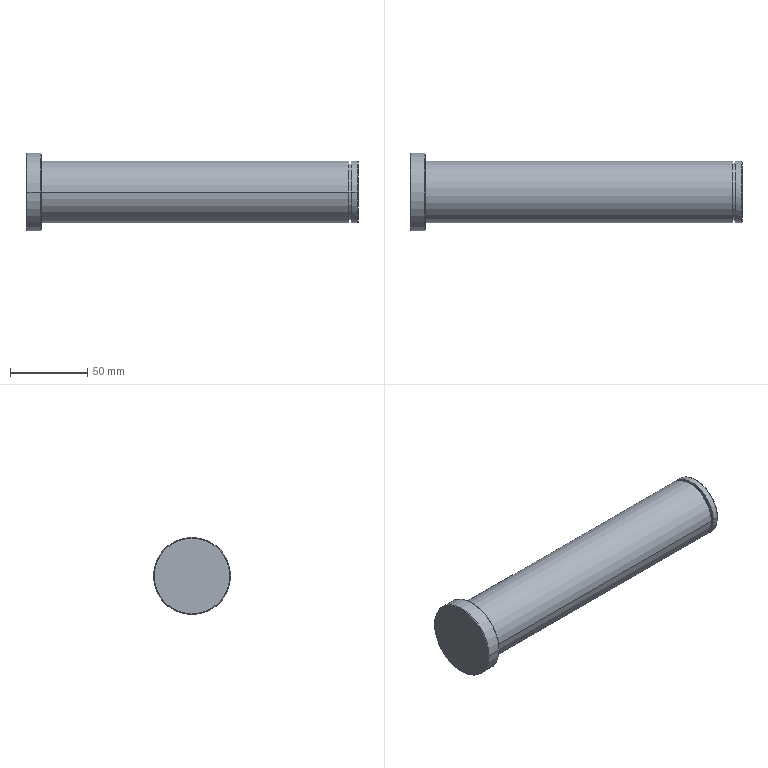Part | SolidWorks | features BaseBody 1 | 1 solid | 19 faces | box 215 x 50 x 50 mm | volume 276823 mm3 | cylinder 8 | cone 6 | plane 5 | commonest cylinder face diameters 40 x4 36.5 x2 50 x2
STEP:
#1=CARTESIAN_POINT('',(24.077,-7.842,0.));
#2=VERTEX_POINT('',#1);
#3=CARTESIAN_POINT('',(24.077,-47.842,0.));
#4=VERTEX_POINT('',#3);
#5=CARTESIAN_POINT('',(24.077,-27.842,0.));
#6=DIRECTION('',(1.,0.,0.));
#7=DIRECTION('',(0.,1.,0.));
#8=AXIS2_PLACEMENT_3D('',#5,#6,#7);
#9=CIRCLE('',#8,20.);
#10=EDGE_CURVE('',#2,#4,#9,.T.);
#11=ORIENTED_EDGE('',*,*,#10,.T.);
#12=CARTESIAN_POINT('',(223.077,-47.842,0.));
#13=VERTEX_POINT('',#12);
#14=CARTESIAN_POINT('',(123.577,-47.842,0.));
#15=DIRECTION('',(1.,0.,0.));
#16=VECTOR('',#15,1000.);
#17=LINE('',#14,#16);
#18=EDGE_CURVE('',#4,#13,#17,.T.);
#19=ORIENTED_EDGE('',*,*,#18,.T.);
#20=CARTESIAN_POINT('',(223.077,-7.842,0.));
#21=VERTEX_POINT('',#20);
#22=CARTESIAN_POINT('',(223.077,-27.842,0.));
#23=DIRECTION('',(-1.,0.,0.));
#24=DIRECTION('',(0.,1.,0.));
#25=AXIS2_PLACEMENT_3D('',#22,#23,#24);
#26=CIRCLE('',#25,20.);
#27=EDGE_CURVE('',#13,#21,#26,.T.);
#28=ORIENTED_EDGE('',*,*,#27,.T.);
#29=CARTESIAN_POINT('',(123.577,-7.842,0.));
#30=DIRECTION('',(1.,0.,0.));
#31=VECTOR('',#30,1000.);
#32=LINE('',#29,#31);
#33=EDGE_CURVE('',#2,#21,#32,.T.);
#34=ORIENTED_EDGE('',*,*,#33,.F.);
#35=EDGE_LOOP('',(#11,#19,#28,#34));
#36=FACE_OUTER_BOUND('',#35,.T.);
#37=CARTESIAN_POINT('',(123.577,-27.842,0.));
#38=DIRECTION('',(1.,0.,0.));
#39=DIRECTION('',(0.,1.,0.));
#40=AXIS2_PLACEMENT_3D('',#37,#38,#39);
#41=CYLINDRICAL_SURFACE('',#40,20.);
#42=ADVANCED_FACE('',(#36),#41,.T.);
#43=CARTESIAN_POINT('',(24.077,-27.842,-24.5));
#44=VERTEX_POINT('',#43);
#45=CARTESIAN_POINT('',(24.077,-27.842,24.5));
#46=VERTEX_POINT('',#45);
#47=CARTESIAN_POINT('',(24.077,-27.842,0.));
#48=DIRECTION('',(1.,0.,0.));
#49=DIRECTION('',(0.,0.,1.));
#50=AXIS2_PLACEMENT_3D('',#47,#48,#49);
#51=CIRCLE('',#50,24.5);
#52=EDGE_CURVE('',#44,#46,#51,.T.);
#53=ORIENTED_EDGE('',*,*,#52,.F.);
#54=CARTESIAN_POINT('',(23.577,-27.842,-25.));
#55=VERTEX_POINT('',#54);
#56=CARTESIAN_POINT('',(23.577,-27.842,-25.));
#57=DIRECTION('',(-0.7071,0.,-0.7071));
#58=VECTOR('',#57,1000.);
#59=LINE('',#56,#58);
#60=EDGE_CURVE('',#44,#55,#59,.T.);
#61=ORIENTED_EDGE('',*,*,#60,.T.);
#62=CARTESIAN_POINT('',(23.577,-2.842,0.));
#63=VERTEX_POINT('',#62);
#64=CARTESIAN_POINT('',(23.577,-27.842,0.));
#65=DIRECTION('',(1.,0.,0.));
#66=DIRECTION('',(0.,-1.,0.));
#67=AXIS2_PLACEMENT_3D('',#64,#65,#66);
#68=CIRCLE('',#67,25.);
#69=EDGE_CURVE('',#55,#63,#68,.T.);
#70=ORIENTED_EDGE('',*,*,#69,.T.);
#71=CARTESIAN_POINT('',(23.577,-27.842,25.));
#72=VERTEX_POINT('',#71);
#73=CARTESIAN_POINT('',(23.577,-27.842,0.));
#74=DIRECTION('',(1.,0.,0.));
#75=DIRECTION('',(0.,-1.,0.));
#76=AXIS2_PLACEMENT_3D('',#73,#74,#75);
#77=CIRCLE('',#76,25.);
#78=EDGE_CURVE('',#63,#72,#77,.T.);
#79=ORIENTED_EDGE('',*,*,#78,.T.);
#80=CARTESIAN_POINT('',(23.577,-27.842,25.));
#81=DIRECTION('',(-0.7071,0.,0.7071));
#82=VECTOR('',#81,1000.);
#83=LINE('',#80,#82);
#84=EDGE_CURVE('',#46,#72,#83,.T.);
#85=ORIENTED_EDGE('',*,*,#84,.F.);
#86=EDGE_LOOP('',(#53,#61,#70,#79,#85));
#87=FACE_OUTER_BOUND('',#86,.T.);
#88=CARTESIAN_POINT('',(23.577,-27.842,0.));
#89=DIRECTION('',(-1.,0.,0.));
#90=DIRECTION('',(0.,0.,1.));
#91=AXIS2_PLACEMENT_3D('',#88,#89,#90);
#92=CONICAL_SURFACE('',#91,25.,0.7854);
#93=ADVANCED_FACE('',(#87),#92,.T.);
#94=CARTESIAN_POINT('',(223.077,-46.092,0.));
#95=VERTEX_POINT('',#94);
#96=CARTESIAN_POINT('',(223.077,-9.592,0.));
#97=VERTEX_POINT('',#96);
#98=CARTESIAN_POINT('',(223.077,-27.842,0.));
#99=DIRECTION('',(-1.,0.,0.));
#100=DIRECTION('',(0.,1.,0.));
#101=AXIS2_PLACEMENT_3D('',#98,#99,#100);
#102=CIRCLE('',#101,18.25);
#103=EDGE_CURVE('',#95,#97,#102,.T.);
#104=ORIENTED_EDGE('',*,*,#103,.F.);
#105=CARTESIAN_POINT('',(224.827,-46.092,0.));
#106=VERTEX_POINT('',#105);
#107=CARTESIAN_POINT('',(223.952,-46.092,0.));
#108=DIRECTION('',(1.,0.,0.));
#109=VECTOR('',#108,1000.);
#110=LINE('',#107,#109);
#111=EDGE_CURVE('',#95,#106,#110,.T.);
#112=ORIENTED_EDGE('',*,*,#111,.T.);
#113=CARTESIAN_POINT('',(224.827,-9.592,0.));
#114=VERTEX_POINT('',#113);
#115=CARTESIAN_POINT('',(224.827,-27.842,0.));
#116=DIRECTION('',(-1.,0.,0.));
#117=DIRECTION('',(0.,1.,0.));
#118=AXIS2_PLACEMENT_3D('',#115,#116,#117);
#119=CIRCLE('',#118,18.25);
#120=EDGE_CURVE('',#106,#114,#119,.T.);
#121=ORIENTED_EDGE('',*,*,#120,.T.);
#122=CARTESIAN_POINT('',(223.952,-9.592,0.));
#123=DIRECTION('',(1.,0.,0.));
#124=VECTOR('',#123,1000.);
#125=LINE('',#122,#124);
#126=EDGE_CURVE('',#97,#114,#125,.T.);
#127=ORIENTED_EDGE('',*,*,#126,.F.);
#128=EDGE_LOOP('',(#104,#112,#121,#127));
#129=FACE_OUTER_BOUND('',#128,.T.);
#130=CARTESIAN_POINT('',(223.952,-27.842,0.));
#131=DIRECTION('',(1.,0.,0.));
#132=DIRECTION('',(0.,1.,0.));
#133=AXIS2_PLACEMENT_3D('',#130,#131,#132);
#134=CYLINDRICAL_SURFACE('',#133,18.25);
#135=ADVANCED_FACE('',(#129),#134,.T.);
#136=CARTESIAN_POINT('',(14.577,-27.842,25.));
#137=VERTEX_POINT('',#136);
#138=CARTESIAN_POINT('',(14.577,-52.842,0.));
#139=VERTEX_POINT('',#138);
#140=CARTESIAN_POINT('',(14.577,-27.842,0.));
#141=DIRECTION('',(1.,0.,0.));
#142=DIRECTION('',(0.,1.,0.));
#143=AXIS2_PLACEMENT_3D('',#140,#141,#142);
#144=CIRCLE('',#143,25.);
#145=EDGE_CURVE('',#137,#139,#144,.T.);
#146=ORIENTED_EDGE('',*,*,#145,.T.);
#147=CARTESIAN_POINT('',(23.577,-52.842,0.));
#148=VERTEX_POINT('',#147);
#149=CARTESIAN_POINT('',(19.077,-52.842,0.));
#150=DIRECTION('',(1.,0.,0.));
#151=VECTOR('',#150,1000.);
#152=LINE('',#149,#151);
#153=EDGE_CURVE('',#139,#148,#152,.T.);
#154=ORIENTED_EDGE('',*,*,#153,.T.);
#155=CARTESIAN_POINT('',(23.577,-27.842,0.));
#156=DIRECTION('',(1.,0.,0.));
#157=DIRECTION('',(0.,-1.,0.));
#158=AXIS2_PLACEMENT_3D('',#155,#156,#157);
#159=CIRCLE('',#158,25.);
#160=EDGE_CURVE('',#72,#148,#159,.T.);
#161=ORIENTED_EDGE('',*,*,#160,.F.);
#162=ORIENTED_EDGE('',*,*,#78,.F.);
#163=CARTESIAN_POINT('',(14.577,-2.842,0.));
#164=VERTEX_POINT('',#163);
#165=CARTESIAN_POINT('',(19.077,-2.842,0.));
#166=DIRECTION('',(1.,0.,0.));
#167=VECTOR('',#166,1000.);
#168=LINE('',#165,#167);
#169=EDGE_CURVE('',#164,#63,#168,.T.);
#170=ORIENTED_EDGE('',*,*,#169,.F.);
#171=CARTESIAN_POINT('',(14.577,-27.842,0.));
#172=DIRECTION('',(1.,0.,0.));
#173=DIRECTION('',(0.,1.,0.));
#174=AXIS2_PLACEMENT_3D('',#171,#172,#173);
#175=CIRCLE('',#174,25.);
#176=EDGE_CURVE('',#164,#137,#175,.T.);
#177=ORIENTED_EDGE('',*,*,#176,.T.);
#178=EDGE_LOOP('',(#146,#154,#161,#162,#170,#177));
#179=FACE_OUTER_BOUND('',#178,.T.);
#180=CARTESIAN_POINT('',(19.077,-27.842,0.));
#181=DIRECTION('',(1.,0.,0.));
#182=DIRECTION('',(0.,1.,0.));
#183=AXIS2_PLACEMENT_3D('',#180,#181,#182);
#184=CYLINDRICAL_SURFACE('',#183,25.);
#185=ADVANCED_FACE('',(#179),#184,.T.);
#186=CARTESIAN_POINT('',(14.077,-27.842,-24.5));
#187=VERTEX_POINT('',#186);
#188=CARTESIAN_POINT('',(14.077,-27.842,24.5));
#189=VERTEX_POINT('',#188);
#190=CARTESIAN_POINT('',(14.077,-27.842,0.));
#191=DIRECTION('',(1.,0.,0.));
#192=DIRECTION('',(0.,0.,-1.));
#193=AXIS2_PLACEMENT_3D('',#190,#191,#192);
#194=CIRCLE('',#193,24.5);
#195=EDGE_CURVE('',#187,#189,#194,.T.);
#196=ORIENTED_EDGE('',*,*,#195,.T.);
#197=CARTESIAN_POINT('',(14.577,-27.842,25.));
#198=DIRECTION('',(0.7071,0.,0.7071));
#199=VECTOR('',#198,1000.);
#200=LINE('',#197,#199);
#201=EDGE_CURVE('',#189,#137,#200,.T.);
#202=ORIENTED_EDGE('',*,*,#201,.T.);
#203=ORIENTED_EDGE('',*,*,#176,.F.);
#204=CARTESIAN_POINT('',(14.577,-27.842,-25.));
#205=VERTEX_POINT('',#204);
#206=CARTESIAN_POINT('',(14.577,-27.842,0.));
#207=DIRECTION('',(1.,0.,0.));
#208=DIRECTION('',(0.,1.,0.));
#209=AXIS2_PLACEMENT_3D('',#206,#207,#208);
#210=CIRCLE('',#209,25.);
#211=EDGE_CURVE('',#205,#164,#210,.T.);
#212=ORIENTED_EDGE('',*,*,#211,.F.);
#213=CARTESIAN_POINT('',(14.577,-27.842,-25.));
#214=DIRECTION('',(0.7071,0.,-0.7071));
#215=VECTOR('',#214,1000.);
#216=LINE('',#213,#215);
#217=EDGE_CURVE('',#187,#205,#216,.T.);
#218=ORIENTED_EDGE('',*,*,#217,.F.);
#219=EDGE_LOOP('',(#196,#202,#203,#212,#218));
#220=FACE_OUTER_BOUND('',#219,.T.);
#221=CARTESIAN_POINT('',(14.577,-27.842,0.));
#222=DIRECTION('',(1.,0.,0.));
#223=DIRECTION('',(0.,0.,-1.));
#224=AXIS2_PLACEMENT_3D('',#221,#222,#223);
#225=CONICAL_SURFACE('',#224,25.,0.7854);
#226=ADVANCED_FACE('',(#220),#225,.T.);
#227=CARTESIAN_POINT('',(224.827,-47.842,0.));
#228=VERTEX_POINT('',#227);
#229=CARTESIAN_POINT('',(224.827,-7.842,0.));
#230=VERTEX_POINT('',#229);
#231=CARTESIAN_POINT('',(224.827,-27.842,0.));
#232=DIRECTION('',(-1.,0.,0.));
#233=DIRECTION('',(0.,1.,0.));
#234=AXIS2_PLACEMENT_3D('',#231,#232,#233);
#235=CIRCLE('',#234,20.);
#236=EDGE_CURVE('',#228,#230,#235,.T.);
#237=ORIENTED_EDGE('',*,*,#236,.F.);
#238=CARTESIAN_POINT('',(228.577,-47.842,0.));
#239=VERTEX_POINT('',#238);
#240=CARTESIAN_POINT('',(226.702,-47.842,0.));
#241=DIRECTION('',(1.,0.,0.));
#242=VECTOR('',#241,1000.);
#243=LINE('',#240,#242);
#244=EDGE_CURVE('',#228,#239,#243,.T.);
#245=ORIENTED_EDGE('',*,*,#244,.T.);
#246=CARTESIAN_POINT('',(228.577,-27.842,20.));
#247=VERTEX_POINT('',#246);
#248=CARTESIAN_POINT('',(228.577,-27.842,0.));
#249=DIRECTION('',(-1.,0.,0.));
#250=DIRECTION('',(0.,1.,0.));
#251=AXIS2_PLACEMENT_3D('',#248,#249,#250);
#252=CIRCLE('',#251,20.);
#253=EDGE_CURVE('',#239,#247,#252,.T.);
#254=ORIENTED_EDGE('',*,*,#253,.T.);
#255=CARTESIAN_POINT('',(228.577,-7.842,0.));
#256=VERTEX_POINT('',#255);
#257=CARTESIAN_POINT('',(228.577,-27.842,0.));
#258=DIRECTION('',(-1.,0.,0.));
#259=DIRECTION('',(0.,1.,0.));
#260=AXIS2_PLACEMENT_3D('',#257,#258,#259);
#261=CIRCLE('',#260,20.);
#262=EDGE_CURVE('',#247,#256,#261,.T.);
#263=ORIENTED_EDGE('',*,*,#262,.T.);
#264=CARTESIAN_POINT('',(226.702,-7.842,0.));
#265=DIRECTION('',(1.,0.,0.));
#266=VECTOR('',#265,1000.);
#267=LINE('',#264,#266);
#268=EDGE_CURVE('',#230,#256,#267,.T.);
#269=ORIENTED_EDGE('',*,*,#268,.F.);
#270=EDGE_LOOP('',(#237,#245,#254,#263,#269));
#271=FACE_OUTER_BOUND('',#270,.T.);
#272=CARTESIAN_POINT('',(226.702,-27.842,0.));
#273=DIRECTION('',(1.,0.,0.));
#274=DIRECTION('',(0.,1.,0.));
#275=AXIS2_PLACEMENT_3D('',#272,#273,#274);
#276=CYLINDRICAL_SURFACE('',#275,20.);
#277=ADVANCED_FACE('',(#271),#276,.T.);
#278=CARTESIAN_POINT('',(229.077,-27.842,19.5));
#279=VERTEX_POINT('',#278);
#280=CARTESIAN_POINT('',(229.077,-27.842,-19.5));
#281=VERTEX_POINT('',#280);
#282=CARTESIAN_POINT('',(229.077,-27.842,0.));
#283=DIRECTION('',(-1.,0.,0.));
#284=DIRECTION('',(0.,0.,1.));
#285=AXIS2_PLACEMENT_3D('',#282,#283,#284);
#286=CIRCLE('',#285,19.5);
#287=EDGE_CURVE('',#279,#281,#286,.T.);
#288=ORIENTED_EDGE('',*,*,#287,.T.);
#289=CARTESIAN_POINT('',(228.577,-27.842,-20.));
#290=VERTEX_POINT('',#289);
#291=CARTESIAN_POINT('',(228.577,-27.842,-20.));
#292=DIRECTION('',(-0.7071,0.,-0.7071));
#293=VECTOR('',#292,1000.);
#294=LINE('',#291,#293);
#295=EDGE_CURVE('',#281,#290,#294,.T.);
#296=ORIENTED_EDGE('',*,*,#295,.T.);
#297=CARTESIAN_POINT('',(228.577,-27.842,0.));
#298=DIRECTION('',(-1.,0.,0.));
#299=DIRECTION('',(0.,1.,0.));
#300=AXIS2_PLACEMENT_3D('',#297,#298,#299);
#301=CIRCLE('',#300,20.);
#302=EDGE_CURVE('',#256,#290,#301,.T.);
#303=ORIENTED_EDGE('',*,*,#302,.F.);
#304=ORIENTED_EDGE('',*,*,#262,.F.);
#305=CARTESIAN_POINT('',(228.577,-27.842,20.));
#306=DIRECTION('',(-0.7071,0.,0.7071));
#307=VECTOR('',#306,1000.);
#308=LINE('',#305,#307);
#309=EDGE_CURVE('',#279,#247,#308,.T.);
#310=ORIENTED_EDGE('',*,*,#309,.F.);
#311=EDGE_LOOP('',(#288,#296,#303,#304,#310));
#312=FACE_OUTER_BOUND('',#311,.T.);
#313=CARTESIAN_POINT('',(228.577,-27.842,0.));
#314=DIRECTION('',(-1.,0.,0.));
#315=DIRECTION('',(0.,0.,1.));
#316=AXIS2_PLACEMENT_3D('',#313,#314,#315);
#317=CONICAL_SURFACE('',#316,20.,0.7854);
#318=ADVANCED_FACE('',(#312),#317,.T.);
#319=ORIENTED_EDGE('',*,*,#18,.F.);
#320=CARTESIAN_POINT('',(24.077,-27.842,0.));
#321=DIRECTION('',(1.,0.,0.));
#322=DIRECTION('',(0.,1.,0.));
#323=AXIS2_PLACEMENT_3D('',#320,#321,#322);
#324=CIRCLE('',#323,20.);
#325=EDGE_CURVE('',#4,#2,#324,.T.);
#326=ORIENTED_EDGE('',*,*,#325,.T.);
#327=ORIENTED_EDGE('',*,*,#33,.T.);
#328=CARTESIAN_POINT('',(223.077,-27.842,0.));
#329=DIRECTION('',(-1.,0.,0.));
#330=DIRECTION('',(0.,1.,0.));
#331=AXIS2_PLACEMENT_3D('',#328,#329,#330);
#332=CIRCLE('',#331,20.);
#333=EDGE_CURVE('',#21,#13,#332,.T.);
#334=ORIENTED_EDGE('',*,*,#333,.T.);
#335=EDGE_LOOP('',(#319,#326,#327,#334));
#336=FACE_OUTER_BOUND('',#335,.T.);
#337=CARTESIAN_POINT('',(123.577,-27.842,0.));
#338=DIRECTION('',(1.,0.,0.));
#339=DIRECTION('',(0.,1.,0.));
#340=AXIS2_PLACEMENT_3D('',#337,#338,#339);
#341=CYLINDRICAL_SURFACE('',#340,20.);
#342=ADVANCED_FACE('',(#336),#341,.T.);
#343=ORIENTED_EDGE('',*,*,#10,.F.);
#344=ORIENTED_EDGE('',*,*,#325,.F.);
#345=EDGE_LOOP('',(#343,#344));
#346=FACE_BOUND('',#345,.T.);
#347=CARTESIAN_POINT('',(24.077,-27.842,0.));
#348=DIRECTION('',(1.,0.,0.));
#349=DIRECTION('',(0.,0.,1.));
#350=AXIS2_PLACEMENT_3D('',#347,#348,#349);
#351=CIRCLE('',#350,24.5);
#352=EDGE_CURVE('',#46,#44,#351,.T.);
#353=ORIENTED_EDGE('',*,*,#352,.T.);
#354=ORIENTED_EDGE('',*,*,#52,.T.);
#355=EDGE_LOOP('',(#353,#354));
#356=FACE_OUTER_BOUND('',#355,.T.);
#357=CARTESIAN_POINT('',(24.077,-5.342,0.));
#358=DIRECTION('',(1.,0.,0.));
#359=DIRECTION('',(0.,1.,0.));
#360=AXIS2_PLACEMENT_3D('',#357,#358,#359);
#361=PLANE('',#360);
#362=ADVANCED_FACE('',(#346,#356),#361,.T.);
#363=CARTESIAN_POINT('',(223.077,-27.842,0.));
#364=DIRECTION('',(-1.,0.,0.));
#365=DIRECTION('',(0.,1.,0.));
#366=AXIS2_PLACEMENT_3D('',#363,#364,#365);
#367=CIRCLE('',#366,18.25);
#368=EDGE_CURVE('',#97,#95,#367,.T.);
#369=ORIENTED_EDGE('',*,*,#368,.T.);
#370=ORIENTED_EDGE('',*,*,#103,.T.);
#371=EDGE_LOOP('',(#369,#370));
#372=FACE_BOUND('',#371,.T.);
#373=ORIENTED_EDGE('',*,*,#333,.F.);
#374=ORIENTED_EDGE('',*,*,#27,.F.);
#375=EDGE_LOOP('',(#373,#374));
#376=FACE_OUTER_BOUND('',#375,.T.);
#377=CARTESIAN_POINT('',(223.077,-8.717,0.));
#378=DIRECTION('',(1.,0.,0.));
#379=DIRECTION('',(0.,1.,0.));
#380=AXIS2_PLACEMENT_3D('',#377,#378,#379);
#381=PLANE('',#380);
#382=ADVANCED_FACE('',(#372,#376),#381,.T.);
#383=ORIENTED_EDGE('',*,*,#60,.F.);
#384=ORIENTED_EDGE('',*,*,#352,.F.);
#385=ORIENTED_EDGE('',*,*,#84,.T.);
#386=ORIENTED_EDGE('',*,*,#160,.T.);
#387=CARTESIAN_POINT('',(23.577,-27.842,0.));
#388=DIRECTION('',(1.,0.,0.));
#389=DIRECTION('',(0.,-1.,0.));
#390=AXIS2_PLACEMENT_3D('',#387,#388,#389);
#391=CIRCLE('',#390,25.);
#392=EDGE_CURVE('',#148,#55,#391,.T.);
#393=ORIENTED_EDGE('',*,*,#392,.T.);
#394=EDGE_LOOP('',(#383,#384,#385,#386,#393));
#395=FACE_OUTER_BOUND('',#394,.T.);
#396=CARTESIAN_POINT('',(23.577,-27.842,0.));
#397=DIRECTION('',(-1.,0.,0.));
#398=DIRECTION('',(0.,0.,1.));
#399=AXIS2_PLACEMENT_3D('',#396,#397,#398);
#400=CONICAL_SURFACE('',#399,25.,0.7854);
#401=ADVANCED_FACE('',(#395),#400,.T.);
#402=ORIENTED_EDGE('',*,*,#111,.F.);
#403=ORIENTED_EDGE('',*,*,#368,.F.);
#404=ORIENTED_EDGE('',*,*,#126,.T.);
#405=CARTESIAN_POINT('',(224.827,-27.842,0.));
#406=DIRECTION('',(-1.,0.,0.));
#407=DIRECTION('',(0.,1.,0.));
#408=AXIS2_PLACEMENT_3D('',#405,#406,#407);
#409=CIRCLE('',#408,18.25);
#410=EDGE_CURVE('',#114,#106,#409,.T.);
#411=ORIENTED_EDGE('',*,*,#410,.T.);
#412=EDGE_LOOP('',(#402,#403,#404,#411));
#413=FACE_OUTER_BOUND('',#412,.T.);
#414=CARTESIAN_POINT('',(223.952,-27.842,0.));
#415=DIRECTION('',(1.,0.,0.));
#416=DIRECTION('',(0.,1.,0.));
#417=AXIS2_PLACEMENT_3D('',#414,#415,#416);
#418=CYLINDRICAL_SURFACE('',#417,18.25);
#419=ADVANCED_FACE('',(#413),#418,.T.);
#420=ORIENTED_EDGE('',*,*,#153,.F.);
#421=CARTESIAN_POINT('',(14.577,-27.842,0.));
#422=DIRECTION('',(1.,0.,0.));
#423=DIRECTION('',(0.,1.,0.));
#424=AXIS2_PLACEMENT_3D('',#421,#422,#423);
#425=CIRCLE('',#424,25.);
#426=EDGE_CURVE('',#139,#205,#425,.T.);
#427=ORIENTED_EDGE('',*,*,#426,.T.);
#428=ORIENTED_EDGE('',*,*,#211,.T.);
#429=ORIENTED_EDGE('',*,*,#169,.T.);
#430=ORIENTED_EDGE('',*,*,#69,.F.);
#431=ORIENTED_EDGE('',*,*,#392,.F.);
#432=EDGE_LOOP('',(#420,#427,#428,#429,#430,#431));
#433=FACE_OUTER_BOUND('',#432,.T.);
#434=CARTESIAN_POINT('',(19.077,-27.842,0.));
#435=DIRECTION('',(1.,0.,0.));
#436=DIRECTION('',(0.,1.,0.));
#437=AXIS2_PLACEMENT_3D('',#434,#435,#436);
#438=CYLINDRICAL_SURFACE('',#437,25.);
#439=ADVANCED_FACE('',(#433),#438,.T.);
#440=ORIENTED_EDGE('',*,*,#410,.F.);
#441=ORIENTED_EDGE('',*,*,#120,.F.);
#442=EDGE_LOOP('',(#440,#441));
#443=FACE_BOUND('',#442,.T.);
#444=CARTESIAN_POINT('',(224.827,-27.842,0.));
#445=DIRECTION('',(-1.,0.,0.));
#446=DIRECTION('',(0.,1.,0.));
#447=AXIS2_PLACEMENT_3D('',#444,#445,#446);
#448=CIRCLE('',#447,20.);
#449=EDGE_CURVE('',#230,#228,#448,.T.);
#450=ORIENTED_EDGE('',*,*,#449,.T.);
#451=ORIENTED_EDGE('',*,*,#236,.T.);
#452=EDGE_LOOP('',(#450,#451));
#453=FACE_OUTER_BOUND('',#452,.T.);
#454=CARTESIAN_POINT('',(224.827,-8.717,0.));
#455=DIRECTION('',(-1.,0.,0.));
#456=DIRECTION('',(0.,-1.,0.));
#457=AXIS2_PLACEMENT_3D('',#454,#455,#456);
#458=PLANE('',#457);
#459=ADVANCED_FACE('',(#443,#453),#458,.T.);
#460=ORIENTED_EDGE('',*,*,#201,.F.);
#461=CARTESIAN_POINT('',(14.077,-27.842,0.));
#462=DIRECTION('',(1.,0.,0.));
#463=DIRECTION('',(0.,0.,-1.));
#464=AXIS2_PLACEMENT_3D('',#461,#462,#463);
#465=CIRCLE('',#464,24.5);
#466=EDGE_CURVE('',#189,#187,#465,.T.);
#467=ORIENTED_EDGE('',*,*,#466,.T.);
#468=ORIENTED_EDGE('',*,*,#217,.T.);
#469=ORIENTED_EDGE('',*,*,#426,.F.);
#470=ORIENTED_EDGE('',*,*,#145,.F.);
#471=EDGE_LOOP('',(#460,#467,#468,#469,#470));
#472=FACE_OUTER_BOUND('',#471,.T.);
#473=CARTESIAN_POINT('',(14.577,-27.842,0.));
#474=DIRECTION('',(1.,0.,0.));
#475=DIRECTION('',(0.,0.,-1.));
#476=AXIS2_PLACEMENT_3D('',#473,#474,#475);
#477=CONICAL_SURFACE('',#476,25.,0.7854);
#478=ADVANCED_FACE('',(#472),#477,.T.);
#479=ORIENTED_EDGE('',*,*,#244,.F.);
#480=ORIENTED_EDGE('',*,*,#449,.F.);
#481=ORIENTED_EDGE('',*,*,#268,.T.);
#482=ORIENTED_EDGE('',*,*,#302,.T.);
#483=CARTESIAN_POINT('',(228.577,-27.842,0.));
#484=DIRECTION('',(-1.,0.,0.));
#485=DIRECTION('',(0.,1.,0.));
#486=AXIS2_PLACEMENT_3D('',#483,#484,#485);
#487=CIRCLE('',#486,20.);
#488=EDGE_CURVE('',#290,#239,#487,.T.);
#489=ORIENTED_EDGE('',*,*,#488,.T.);
#490=EDGE_LOOP('',(#479,#480,#481,#482,#489));
#491=FACE_OUTER_BOUND('',#490,.T.);
#492=CARTESIAN_POINT('',(226.702,-27.842,0.));
#493=DIRECTION('',(1.,0.,0.));
#494=DIRECTION('',(0.,1.,0.));
#495=AXIS2_PLACEMENT_3D('',#492,#493,#494);
#496=CYLINDRICAL_SURFACE('',#495,20.);
#497=ADVANCED_FACE('',(#491),#496,.T.);
#498=ORIENTED_EDGE('',*,*,#195,.F.);
#499=ORIENTED_EDGE('',*,*,#466,.F.);
#500=EDGE_LOOP('',(#498,#499));
#501=FACE_OUTER_BOUND('',#500,.T.);
#502=CARTESIAN_POINT('',(14.077,-15.342,0.));
#503=DIRECTION('',(-1.,0.,0.));
#504=DIRECTION('',(0.,-1.,0.));
#505=AXIS2_PLACEMENT_3D('',#502,#503,#504);
#506=PLANE('',#505);
#507=ADVANCED_FACE('',(#501),#506,.T.);
#508=ORIENTED_EDGE('',*,*,#295,.F.);
#509=CARTESIAN_POINT('',(229.077,-27.842,0.));
#510=DIRECTION('',(-1.,0.,0.));
#511=DIRECTION('',(0.,0.,1.));
#512=AXIS2_PLACEMENT_3D('',#509,#510,#511);
#513=CIRCLE('',#512,19.5);
#514=EDGE_CURVE('',#281,#279,#513,.T.);
#515=ORIENTED_EDGE('',*,*,#514,.T.);
#516=ORIENTED_EDGE('',*,*,#309,.T.);
#517=ORIENTED_EDGE('',*,*,#253,.F.);
#518=ORIENTED_EDGE('',*,*,#488,.F.);
#519=EDGE_LOOP('',(#508,#515,#516,#517,#518));
#520=FACE_OUTER_BOUND('',#519,.T.);
#521=CARTESIAN_POINT('',(228.577,-27.842,0.));
#522=DIRECTION('',(-1.,0.,0.));
#523=DIRECTION('',(0.,0.,1.));
#524=AXIS2_PLACEMENT_3D('',#521,#522,#523);
#525=CONICAL_SURFACE('',#524,20.,0.7854);
#526=ADVANCED_FACE('',(#520),#525,.T.);
#527=ORIENTED_EDGE('',*,*,#287,.F.);
#528=ORIENTED_EDGE('',*,*,#514,.F.);
#529=EDGE_LOOP('',(#527,#528));
#530=FACE_OUTER_BOUND('',#529,.T.);
#531=CARTESIAN_POINT('',(229.077,-18.092,0.));
#532=DIRECTION('',(1.,0.,0.));
#533=DIRECTION('',(0.,1.,0.));
#534=AXIS2_PLACEMENT_3D('',#531,#532,#533);
#535=PLANE('',#534);
#536=ADVANCED_FACE('',(#530),#535,.T.);
#537=CLOSED_SHELL('',(#42,#93,#135,#185,#226,#277,#318,#342,#362,#382,#401,#419,#439,#459,#478,#497,#507,#526,#536));
#538=MANIFOLD_SOLID_BREP('',#537);
#539=CARTESIAN_POINT('',(0.,0.,0.));
#540=DIRECTION('',(0.,0.,1.));
#541=DIRECTION('',(1.,0.,0.));
#542=AXIS2_PLACEMENT_3D('',#539,#540,#541);
#543=(LENGTH_UNIT()NAMED_UNIT(*)SI_UNIT(.MILLI.,.METRE.));
#544=UNCERTAINTY_MEASURE_WITH_UNIT(LENGTH_MEASURE(0.00001),#543,'','');
#545=(NAMED_UNIT(*)PLANE_ANGLE_UNIT()SI_UNIT($,.RADIAN.));
#546=(NAMED_UNIT(*)SI_UNIT($,.STERADIAN.)SOLID_ANGLE_UNIT());
#547=(GEOMETRIC_REPRESENTATION_CONTEXT(3)GLOBAL_UNCERTAINTY_ASSIGNED_CONTEXT((#544))GLOBAL_UNIT_ASSIGNED_CONTEXT((#543,#545,#546))REPRESENTATION_CONTEXT('',''));
#548=ADVANCED_BREP_SHAPE_REPRESENTATION('',(#538,#542),#547);